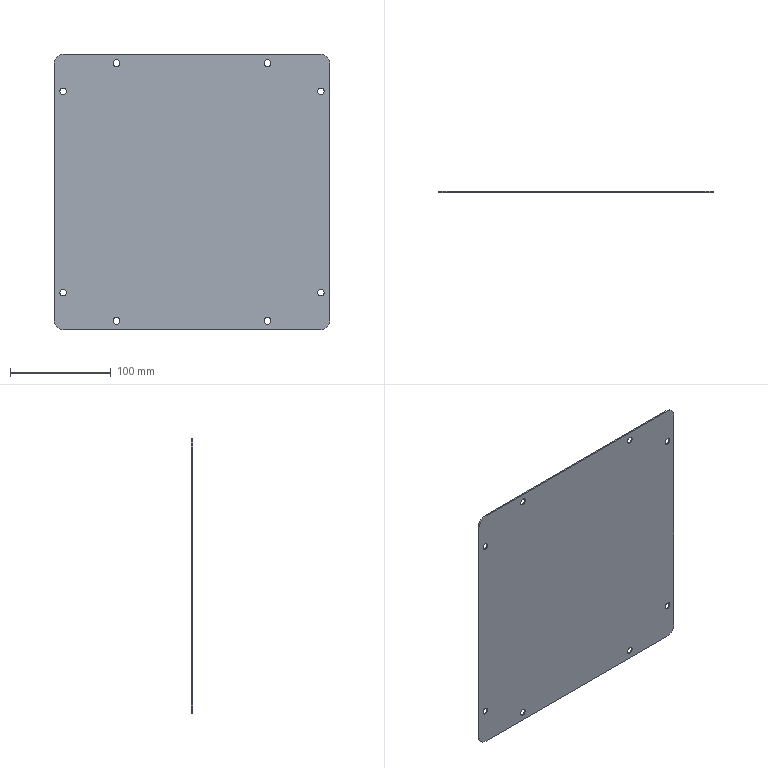Part | STEP file | JBJ-P-1013-05 | 1 solid | 18 faces | box 274 x 1.2 x 274 mm | volume 89670 mm3 | cylinder 12 | plane 6 | commonest cylinder face diameters 6.5 x8 20 x4
STEP:
#1=CARTESIAN_POINT('',(128.,0.,96.75));
#2=VERTEX_POINT('',#1);
#3=CARTESIAN_POINT('',(128.,0.,100.));
#4=DIRECTION('',(0.,-1.,0.));
#5=DIRECTION('',(0.,0.,-1.));
#6=AXIS2_PLACEMENT_3D('',#3,#4,#5);
#7=CIRCLE('',#6,3.25);
#8=EDGE_CURVE('',#2,#2,#7,.T.);
#9=ORIENTED_EDGE('',*,*,#8,.T.);
#10=EDGE_LOOP('',(#9));
#11=FACE_BOUND('',#10,.T.);
#12=CARTESIAN_POINT('',(128.,0.,-103.25));
#13=VERTEX_POINT('',#12);
#14=CARTESIAN_POINT('',(128.,0.,-100.));
#15=DIRECTION('',(0.,-1.,0.));
#16=DIRECTION('',(0.,0.,-1.));
#17=AXIS2_PLACEMENT_3D('',#14,#15,#16);
#18=CIRCLE('',#17,3.25);
#19=EDGE_CURVE('',#13,#13,#18,.T.);
#20=ORIENTED_EDGE('',*,*,#19,.T.);
#21=EDGE_LOOP('',(#20));
#22=FACE_BOUND('',#21,.T.);
#23=CARTESIAN_POINT('',(-128.,0.,-103.25));
#24=VERTEX_POINT('',#23);
#25=CARTESIAN_POINT('',(-128.,0.,-100.));
#26=DIRECTION('',(0.,-1.,0.));
#27=DIRECTION('',(0.,0.,-1.));
#28=AXIS2_PLACEMENT_3D('',#25,#26,#27);
#29=CIRCLE('',#28,3.25);
#30=EDGE_CURVE('',#24,#24,#29,.T.);
#31=ORIENTED_EDGE('',*,*,#30,.T.);
#32=EDGE_LOOP('',(#31));
#33=FACE_BOUND('',#32,.T.);
#34=CARTESIAN_POINT('',(-128.,0.,96.75));
#35=VERTEX_POINT('',#34);
#36=CARTESIAN_POINT('',(-128.,0.,100.));
#37=DIRECTION('',(0.,-1.,0.));
#38=DIRECTION('',(0.,0.,-1.));
#39=AXIS2_PLACEMENT_3D('',#36,#37,#38);
#40=CIRCLE('',#39,3.25);
#41=EDGE_CURVE('',#35,#35,#40,.T.);
#42=ORIENTED_EDGE('',*,*,#41,.T.);
#43=EDGE_LOOP('',(#42));
#44=FACE_BOUND('',#43,.T.);
#45=CARTESIAN_POINT('',(-75.,0.,124.75));
#46=VERTEX_POINT('',#45);
#47=CARTESIAN_POINT('',(-75.,0.,128.));
#48=DIRECTION('',(0.,-1.,0.));
#49=DIRECTION('',(0.,0.,-1.));
#50=AXIS2_PLACEMENT_3D('',#47,#48,#49);
#51=CIRCLE('',#50,3.25);
#52=EDGE_CURVE('',#46,#46,#51,.T.);
#53=ORIENTED_EDGE('',*,*,#52,.T.);
#54=EDGE_LOOP('',(#53));
#55=FACE_BOUND('',#54,.T.);
#56=CARTESIAN_POINT('',(75.,0.,124.75));
#57=VERTEX_POINT('',#56);
#58=CARTESIAN_POINT('',(75.,0.,128.));
#59=DIRECTION('',(0.,-1.,0.));
#60=DIRECTION('',(0.,0.,-1.));
#61=AXIS2_PLACEMENT_3D('',#58,#59,#60);
#62=CIRCLE('',#61,3.25);
#63=EDGE_CURVE('',#57,#57,#62,.T.);
#64=ORIENTED_EDGE('',*,*,#63,.T.);
#65=EDGE_LOOP('',(#64));
#66=FACE_BOUND('',#65,.T.);
#67=CARTESIAN_POINT('',(75.,0.,-131.25));
#68=VERTEX_POINT('',#67);
#69=CARTESIAN_POINT('',(75.,0.,-128.));
#70=DIRECTION('',(0.,-1.,0.));
#71=DIRECTION('',(0.,0.,-1.));
#72=AXIS2_PLACEMENT_3D('',#69,#70,#71);
#73=CIRCLE('',#72,3.25);
#74=EDGE_CURVE('',#68,#68,#73,.T.);
#75=ORIENTED_EDGE('',*,*,#74,.T.);
#76=EDGE_LOOP('',(#75));
#77=FACE_BOUND('',#76,.T.);
#78=CARTESIAN_POINT('',(-127.,0.,137.));
#79=VERTEX_POINT('',#78);
#80=CARTESIAN_POINT('',(127.,0.,137.));
#81=VERTEX_POINT('',#80);
#82=CARTESIAN_POINT('',(-137.,0.,137.));
#83=DIRECTION('',(1.,0.,0.));
#84=VECTOR('',#83,1000.);
#85=LINE('',#82,#84);
#86=EDGE_CURVE('',#79,#81,#85,.T.);
#87=ORIENTED_EDGE('',*,*,#86,.T.);
#88=CARTESIAN_POINT('',(137.,0.,127.));
#89=VERTEX_POINT('',#88);
#90=CARTESIAN_POINT('',(127.,0.,127.));
#91=DIRECTION('',(0.,1.,0.));
#92=DIRECTION('',(0.,0.,1.));
#93=AXIS2_PLACEMENT_3D('',#90,#91,#92);
#94=CIRCLE('',#93,10.);
#95=EDGE_CURVE('',#81,#89,#94,.T.);
#96=ORIENTED_EDGE('',*,*,#95,.T.);
#97=CARTESIAN_POINT('',(137.,0.,-127.));
#98=VERTEX_POINT('',#97);
#99=CARTESIAN_POINT('',(137.,0.,-137.));
#100=DIRECTION('',(0.,0.,-1.));
#101=VECTOR('',#100,1000.);
#102=LINE('',#99,#101);
#103=EDGE_CURVE('',#89,#98,#102,.T.);
#104=ORIENTED_EDGE('',*,*,#103,.T.);
#105=CARTESIAN_POINT('',(127.,0.,-137.));
#106=VERTEX_POINT('',#105);
#107=CARTESIAN_POINT('',(127.,0.,-127.));
#108=DIRECTION('',(0.,1.,0.));
#109=DIRECTION('',(0.,0.,1.));
#110=AXIS2_PLACEMENT_3D('',#107,#108,#109);
#111=CIRCLE('',#110,10.);
#112=EDGE_CURVE('',#98,#106,#111,.T.);
#113=ORIENTED_EDGE('',*,*,#112,.T.);
#114=CARTESIAN_POINT('',(-127.,0.,-137.));
#115=VERTEX_POINT('',#114);
#116=CARTESIAN_POINT('',(-137.,0.,-137.));
#117=DIRECTION('',(-1.,0.,0.));
#118=VECTOR('',#117,1000.);
#119=LINE('',#116,#118);
#120=EDGE_CURVE('',#106,#115,#119,.T.);
#121=ORIENTED_EDGE('',*,*,#120,.T.);
#122=CARTESIAN_POINT('',(-137.,0.,-127.));
#123=VERTEX_POINT('',#122);
#124=CARTESIAN_POINT('',(-127.,0.,-127.));
#125=DIRECTION('',(0.,1.,0.));
#126=DIRECTION('',(0.,0.,1.));
#127=AXIS2_PLACEMENT_3D('',#124,#125,#126);
#128=CIRCLE('',#127,10.);
#129=EDGE_CURVE('',#115,#123,#128,.T.);
#130=ORIENTED_EDGE('',*,*,#129,.T.);
#131=CARTESIAN_POINT('',(-137.,0.,127.));
#132=VERTEX_POINT('',#131);
#133=CARTESIAN_POINT('',(-137.,0.,-137.));
#134=DIRECTION('',(0.,0.,1.));
#135=VECTOR('',#134,1000.);
#136=LINE('',#133,#135);
#137=EDGE_CURVE('',#123,#132,#136,.T.);
#138=ORIENTED_EDGE('',*,*,#137,.T.);
#139=CARTESIAN_POINT('',(-127.,0.,127.));
#140=DIRECTION('',(0.,1.,0.));
#141=DIRECTION('',(0.,0.,1.));
#142=AXIS2_PLACEMENT_3D('',#139,#140,#141);
#143=CIRCLE('',#142,10.);
#144=EDGE_CURVE('',#132,#79,#143,.T.);
#145=ORIENTED_EDGE('',*,*,#144,.T.);
#146=EDGE_LOOP('',(#87,#96,#104,#113,#121,#130,#138,#145));
#147=FACE_OUTER_BOUND('',#146,.T.);
#148=CARTESIAN_POINT('',(-75.,0.,-131.25));
#149=VERTEX_POINT('',#148);
#150=CARTESIAN_POINT('',(-75.,0.,-128.));
#151=DIRECTION('',(0.,-1.,0.));
#152=DIRECTION('',(0.,0.,-1.));
#153=AXIS2_PLACEMENT_3D('',#150,#151,#152);
#154=CIRCLE('',#153,3.25);
#155=EDGE_CURVE('',#149,#149,#154,.T.);
#156=ORIENTED_EDGE('',*,*,#155,.T.);
#157=EDGE_LOOP('',(#156));
#158=FACE_BOUND('',#157,.T.);
#159=CARTESIAN_POINT('',(0.,0.,0.));
#160=DIRECTION('',(0.,1.,0.));
#161=DIRECTION('',(0.,0.,1.));
#162=AXIS2_PLACEMENT_3D('',#159,#160,#161);
#163=PLANE('',#162);
#164=ADVANCED_FACE('',(#11,#22,#33,#44,#55,#66,#77,#147,#158),#163,.T.);
#165=ORIENTED_EDGE('',*,*,#103,.F.);
#166=CARTESIAN_POINT('',(137.,-1.2,127.));
#167=VERTEX_POINT('',#166);
#168=CARTESIAN_POINT('',(137.,-1.2,127.));
#169=DIRECTION('',(0.,-1.,0.));
#170=VECTOR('',#169,1000.);
#171=LINE('',#168,#170);
#172=EDGE_CURVE('',#89,#167,#171,.T.);
#173=ORIENTED_EDGE('',*,*,#172,.T.);
#174=CARTESIAN_POINT('',(137.,-1.2,-127.));
#175=VERTEX_POINT('',#174);
#176=CARTESIAN_POINT('',(137.,-1.2,-137.));
#177=DIRECTION('',(0.,0.,-1.));
#178=VECTOR('',#177,1000.);
#179=LINE('',#176,#178);
#180=EDGE_CURVE('',#167,#175,#179,.T.);
#181=ORIENTED_EDGE('',*,*,#180,.T.);
#182=CARTESIAN_POINT('',(137.,-1.2,-127.));
#183=DIRECTION('',(0.,1.,0.));
#184=VECTOR('',#183,1000.);
#185=LINE('',#182,#184);
#186=EDGE_CURVE('',#175,#98,#185,.T.);
#187=ORIENTED_EDGE('',*,*,#186,.T.);
#188=EDGE_LOOP('',(#165,#173,#181,#187));
#189=FACE_OUTER_BOUND('',#188,.T.);
#190=CARTESIAN_POINT('',(137.,-1.2,-137.));
#191=DIRECTION('',(1.,0.,0.));
#192=DIRECTION('',(0.,0.,-1.));
#193=AXIS2_PLACEMENT_3D('',#190,#191,#192);
#194=PLANE('',#193);
#195=ADVANCED_FACE('',(#189),#194,.T.);
#196=CARTESIAN_POINT('',(-127.,-1.2,137.));
#197=VERTEX_POINT('',#196);
#198=CARTESIAN_POINT('',(127.,-1.2,137.));
#199=VERTEX_POINT('',#198);
#200=CARTESIAN_POINT('',(-137.,-1.2,137.));
#201=DIRECTION('',(1.,0.,0.));
#202=VECTOR('',#201,1000.);
#203=LINE('',#200,#202);
#204=EDGE_CURVE('',#197,#199,#203,.T.);
#205=ORIENTED_EDGE('',*,*,#204,.T.);
#206=CARTESIAN_POINT('',(127.,-1.2,137.));
#207=DIRECTION('',(0.,1.,0.));
#208=VECTOR('',#207,1000.);
#209=LINE('',#206,#208);
#210=EDGE_CURVE('',#199,#81,#209,.T.);
#211=ORIENTED_EDGE('',*,*,#210,.T.);
#212=ORIENTED_EDGE('',*,*,#86,.F.);
#213=CARTESIAN_POINT('',(-127.,-1.2,137.));
#214=DIRECTION('',(0.,-1.,0.));
#215=VECTOR('',#214,1000.);
#216=LINE('',#213,#215);
#217=EDGE_CURVE('',#79,#197,#216,.T.);
#218=ORIENTED_EDGE('',*,*,#217,.T.);
#219=EDGE_LOOP('',(#205,#211,#212,#218));
#220=FACE_OUTER_BOUND('',#219,.T.);
#221=CARTESIAN_POINT('',(-137.,-1.2,137.));
#222=DIRECTION('',(0.,0.,1.));
#223=DIRECTION('',(1.,0.,0.));
#224=AXIS2_PLACEMENT_3D('',#221,#222,#223);
#225=PLANE('',#224);
#226=ADVANCED_FACE('',(#220),#225,.T.);
#227=ORIENTED_EDGE('',*,*,#137,.F.);
#228=CARTESIAN_POINT('',(-137.,-1.2,-127.));
#229=VERTEX_POINT('',#228);
#230=CARTESIAN_POINT('',(-137.,-1.2,-127.));
#231=DIRECTION('',(0.,-1.,0.));
#232=VECTOR('',#231,1000.);
#233=LINE('',#230,#232);
#234=EDGE_CURVE('',#123,#229,#233,.T.);
#235=ORIENTED_EDGE('',*,*,#234,.T.);
#236=CARTESIAN_POINT('',(-137.,-1.2,127.));
#237=VERTEX_POINT('',#236);
#238=CARTESIAN_POINT('',(-137.,-1.2,-137.));
#239=DIRECTION('',(0.,0.,1.));
#240=VECTOR('',#239,1000.);
#241=LINE('',#238,#240);
#242=EDGE_CURVE('',#229,#237,#241,.T.);
#243=ORIENTED_EDGE('',*,*,#242,.T.);
#244=CARTESIAN_POINT('',(-137.,-1.2,127.));
#245=DIRECTION('',(0.,1.,0.));
#246=VECTOR('',#245,1000.);
#247=LINE('',#244,#246);
#248=EDGE_CURVE('',#237,#132,#247,.T.);
#249=ORIENTED_EDGE('',*,*,#248,.T.);
#250=EDGE_LOOP('',(#227,#235,#243,#249));
#251=FACE_OUTER_BOUND('',#250,.T.);
#252=CARTESIAN_POINT('',(-137.,-1.2,-137.));
#253=DIRECTION('',(-1.,0.,0.));
#254=DIRECTION('',(0.,0.,1.));
#255=AXIS2_PLACEMENT_3D('',#252,#253,#254);
#256=PLANE('',#255);
#257=ADVANCED_FACE('',(#251),#256,.T.);
#258=ORIENTED_EDGE('',*,*,#120,.F.);
#259=CARTESIAN_POINT('',(127.,-1.2,-137.));
#260=VERTEX_POINT('',#259);
#261=CARTESIAN_POINT('',(127.,-1.2,-137.));
#262=DIRECTION('',(0.,-1.,0.));
#263=VECTOR('',#262,1000.);
#264=LINE('',#261,#263);
#265=EDGE_CURVE('',#106,#260,#264,.T.);
#266=ORIENTED_EDGE('',*,*,#265,.T.);
#267=CARTESIAN_POINT('',(-127.,-1.2,-137.));
#268=VERTEX_POINT('',#267);
#269=CARTESIAN_POINT('',(-137.,-1.2,-137.));
#270=DIRECTION('',(-1.,0.,0.));
#271=VECTOR('',#270,1000.);
#272=LINE('',#269,#271);
#273=EDGE_CURVE('',#260,#268,#272,.T.);
#274=ORIENTED_EDGE('',*,*,#273,.T.);
#275=CARTESIAN_POINT('',(-127.,-1.2,-137.));
#276=DIRECTION('',(0.,1.,0.));
#277=VECTOR('',#276,1000.);
#278=LINE('',#275,#277);
#279=EDGE_CURVE('',#268,#115,#278,.T.);
#280=ORIENTED_EDGE('',*,*,#279,.T.);
#281=EDGE_LOOP('',(#258,#266,#274,#280));
#282=FACE_OUTER_BOUND('',#281,.T.);
#283=CARTESIAN_POINT('',(-137.,-1.2,-137.));
#284=DIRECTION('',(0.,0.,-1.));
#285=DIRECTION('',(-1.,0.,0.));
#286=AXIS2_PLACEMENT_3D('',#283,#284,#285);
#287=PLANE('',#286);
#288=ADVANCED_FACE('',(#282),#287,.T.);
#289=CARTESIAN_POINT('',(128.,-1.2,96.75));
#290=VERTEX_POINT('',#289);
#291=CARTESIAN_POINT('',(128.,-1.2,100.));
#292=DIRECTION('',(0.,-1.,0.));
#293=DIRECTION('',(0.,0.,-1.));
#294=AXIS2_PLACEMENT_3D('',#291,#292,#293);
#295=CIRCLE('',#294,3.25);
#296=EDGE_CURVE('',#290,#290,#295,.T.);
#297=ORIENTED_EDGE('',*,*,#296,.F.);
#298=EDGE_LOOP('',(#297));
#299=FACE_BOUND('',#298,.T.);
#300=CARTESIAN_POINT('',(128.,-1.2,-103.25));
#301=VERTEX_POINT('',#300);
#302=CARTESIAN_POINT('',(128.,-1.2,-100.));
#303=DIRECTION('',(0.,-1.,0.));
#304=DIRECTION('',(0.,0.,-1.));
#305=AXIS2_PLACEMENT_3D('',#302,#303,#304);
#306=CIRCLE('',#305,3.25);
#307=EDGE_CURVE('',#301,#301,#306,.T.);
#308=ORIENTED_EDGE('',*,*,#307,.F.);
#309=EDGE_LOOP('',(#308));
#310=FACE_BOUND('',#309,.T.);
#311=CARTESIAN_POINT('',(-128.,-1.2,-103.25));
#312=VERTEX_POINT('',#311);
#313=CARTESIAN_POINT('',(-128.,-1.2,-100.));
#314=DIRECTION('',(0.,-1.,0.));
#315=DIRECTION('',(0.,0.,-1.));
#316=AXIS2_PLACEMENT_3D('',#313,#314,#315);
#317=CIRCLE('',#316,3.25);
#318=EDGE_CURVE('',#312,#312,#317,.T.);
#319=ORIENTED_EDGE('',*,*,#318,.F.);
#320=EDGE_LOOP('',(#319));
#321=FACE_BOUND('',#320,.T.);
#322=CARTESIAN_POINT('',(-128.,-1.2,96.75));
#323=VERTEX_POINT('',#322);
#324=CARTESIAN_POINT('',(-128.,-1.2,100.));
#325=DIRECTION('',(0.,-1.,0.));
#326=DIRECTION('',(0.,0.,-1.));
#327=AXIS2_PLACEMENT_3D('',#324,#325,#326);
#328=CIRCLE('',#327,3.25);
#329=EDGE_CURVE('',#323,#323,#328,.T.);
#330=ORIENTED_EDGE('',*,*,#329,.F.);
#331=EDGE_LOOP('',(#330));
#332=FACE_BOUND('',#331,.T.);
#333=CARTESIAN_POINT('',(-75.,-1.2,124.75));
#334=VERTEX_POINT('',#333);
#335=CARTESIAN_POINT('',(-75.,-1.2,128.));
#336=DIRECTION('',(0.,-1.,0.));
#337=DIRECTION('',(0.,0.,-1.));
#338=AXIS2_PLACEMENT_3D('',#335,#336,#337);
#339=CIRCLE('',#338,3.25);
#340=EDGE_CURVE('',#334,#334,#339,.T.);
#341=ORIENTED_EDGE('',*,*,#340,.F.);
#342=EDGE_LOOP('',(#341));
#343=FACE_BOUND('',#342,.T.);
#344=CARTESIAN_POINT('',(75.,-1.2,124.75));
#345=VERTEX_POINT('',#344);
#346=CARTESIAN_POINT('',(75.,-1.2,128.));
#347=DIRECTION('',(0.,-1.,0.));
#348=DIRECTION('',(0.,0.,-1.));
#349=AXIS2_PLACEMENT_3D('',#346,#347,#348);
#350=CIRCLE('',#349,3.25);
#351=EDGE_CURVE('',#345,#345,#350,.T.);
#352=ORIENTED_EDGE('',*,*,#351,.F.);
#353=EDGE_LOOP('',(#352));
#354=FACE_BOUND('',#353,.T.);
#355=CARTESIAN_POINT('',(75.,-1.2,-131.25));
#356=VERTEX_POINT('',#355);
#357=CARTESIAN_POINT('',(75.,-1.2,-128.));
#358=DIRECTION('',(0.,-1.,0.));
#359=DIRECTION('',(0.,0.,-1.));
#360=AXIS2_PLACEMENT_3D('',#357,#358,#359);
#361=CIRCLE('',#360,3.25);
#362=EDGE_CURVE('',#356,#356,#361,.T.);
#363=ORIENTED_EDGE('',*,*,#362,.F.);
#364=EDGE_LOOP('',(#363));
#365=FACE_BOUND('',#364,.T.);
#366=CARTESIAN_POINT('',(-75.,-1.2,-131.25));
#367=VERTEX_POINT('',#366);
#368=CARTESIAN_POINT('',(-75.,-1.2,-128.));
#369=DIRECTION('',(0.,-1.,0.));
#370=DIRECTION('',(0.,0.,-1.));
#371=AXIS2_PLACEMENT_3D('',#368,#369,#370);
#372=CIRCLE('',#371,3.25);
#373=EDGE_CURVE('',#367,#367,#372,.T.);
#374=ORIENTED_EDGE('',*,*,#373,.F.);
#375=EDGE_LOOP('',(#374));
#376=FACE_BOUND('',#375,.T.);
#377=ORIENTED_EDGE('',*,*,#180,.F.);
#378=CARTESIAN_POINT('',(127.,-1.2,127.));
#379=DIRECTION('',(0.,-1.,0.));
#380=DIRECTION('',(0.,0.,1.));
#381=AXIS2_PLACEMENT_3D('',#378,#379,#380);
#382=CIRCLE('',#381,10.);
#383=EDGE_CURVE('',#167,#199,#382,.T.);
#384=ORIENTED_EDGE('',*,*,#383,.T.);
#385=ORIENTED_EDGE('',*,*,#204,.F.);
#386=CARTESIAN_POINT('',(-127.,-1.2,127.));
#387=DIRECTION('',(0.,-1.,0.));
#388=DIRECTION('',(0.,0.,1.));
#389=AXIS2_PLACEMENT_3D('',#386,#387,#388);
#390=CIRCLE('',#389,10.);
#391=EDGE_CURVE('',#197,#237,#390,.T.);
#392=ORIENTED_EDGE('',*,*,#391,.T.);
#393=ORIENTED_EDGE('',*,*,#242,.F.);
#394=CARTESIAN_POINT('',(-127.,-1.2,-127.));
#395=DIRECTION('',(0.,-1.,0.));
#396=DIRECTION('',(0.,0.,1.));
#397=AXIS2_PLACEMENT_3D('',#394,#395,#396);
#398=CIRCLE('',#397,10.);
#399=EDGE_CURVE('',#229,#268,#398,.T.);
#400=ORIENTED_EDGE('',*,*,#399,.T.);
#401=ORIENTED_EDGE('',*,*,#273,.F.);
#402=CARTESIAN_POINT('',(127.,-1.2,-127.));
#403=DIRECTION('',(0.,-1.,0.));
#404=DIRECTION('',(0.,0.,1.));
#405=AXIS2_PLACEMENT_3D('',#402,#403,#404);
#406=CIRCLE('',#405,10.);
#407=EDGE_CURVE('',#260,#175,#406,.T.);
#408=ORIENTED_EDGE('',*,*,#407,.T.);
#409=EDGE_LOOP('',(#377,#384,#385,#392,#393,#400,#401,#408));
#410=FACE_OUTER_BOUND('',#409,.T.);
#411=CARTESIAN_POINT('',(0.,-1.2,0.));
#412=DIRECTION('',(0.,1.,0.));
#413=DIRECTION('',(0.,0.,1.));
#414=AXIS2_PLACEMENT_3D('',#411,#412,#413);
#415=PLANE('',#414);
#416=ADVANCED_FACE('',(#299,#310,#321,#332,#343,#354,#365,#376,#410),#415,.F.);
#417=ORIENTED_EDGE('',*,*,#383,.F.);
#418=ORIENTED_EDGE('',*,*,#172,.F.);
#419=ORIENTED_EDGE('',*,*,#95,.F.);
#420=ORIENTED_EDGE('',*,*,#210,.F.);
#421=EDGE_LOOP('',(#417,#418,#419,#420));
#422=FACE_OUTER_BOUND('',#421,.T.);
#423=CARTESIAN_POINT('',(127.,-1.2,127.));
#424=DIRECTION('',(0.,1.,0.));
#425=DIRECTION('',(0.,0.,1.));
#426=AXIS2_PLACEMENT_3D('',#423,#424,#425);
#427=CYLINDRICAL_SURFACE('',#426,10.);
#428=ADVANCED_FACE('',(#422),#427,.T.);
#429=ORIENTED_EDGE('',*,*,#407,.F.);
#430=ORIENTED_EDGE('',*,*,#265,.F.);
#431=ORIENTED_EDGE('',*,*,#112,.F.);
#432=ORIENTED_EDGE('',*,*,#186,.F.);
#433=EDGE_LOOP('',(#429,#430,#431,#432));
#434=FACE_OUTER_BOUND('',#433,.T.);
#435=CARTESIAN_POINT('',(127.,-1.2,-127.));
#436=DIRECTION('',(0.,1.,0.));
#437=DIRECTION('',(0.,0.,1.));
#438=AXIS2_PLACEMENT_3D('',#435,#436,#437);
#439=CYLINDRICAL_SURFACE('',#438,10.);
#440=ADVANCED_FACE('',(#434),#439,.T.);
#441=ORIENTED_EDGE('',*,*,#399,.F.);
#442=ORIENTED_EDGE('',*,*,#234,.F.);
#443=ORIENTED_EDGE('',*,*,#129,.F.);
#444=ORIENTED_EDGE('',*,*,#279,.F.);
#445=EDGE_LOOP('',(#441,#442,#443,#444));
#446=FACE_OUTER_BOUND('',#445,.T.);
#447=CARTESIAN_POINT('',(-127.,-1.2,-127.));
#448=DIRECTION('',(0.,1.,0.));
#449=DIRECTION('',(0.,0.,1.));
#450=AXIS2_PLACEMENT_3D('',#447,#448,#449);
#451=CYLINDRICAL_SURFACE('',#450,10.);
#452=ADVANCED_FACE('',(#446),#451,.T.);
#453=ORIENTED_EDGE('',*,*,#391,.F.);
#454=ORIENTED_EDGE('',*,*,#217,.F.);
#455=ORIENTED_EDGE('',*,*,#144,.F.);
#456=ORIENTED_EDGE('',*,*,#248,.F.);
#457=EDGE_LOOP('',(#453,#454,#455,#456));
#458=FACE_OUTER_BOUND('',#457,.T.);
#459=CARTESIAN_POINT('',(-127.,-1.2,127.));
#460=DIRECTION('',(0.,1.,0.));
#461=DIRECTION('',(0.,0.,1.));
#462=AXIS2_PLACEMENT_3D('',#459,#460,#461);
#463=CYLINDRICAL_SURFACE('',#462,10.);
#464=ADVANCED_FACE('',(#458),#463,.T.);
#465=ORIENTED_EDGE('',*,*,#155,.F.);
#466=EDGE_LOOP('',(#465));
#467=FACE_OUTER_BOUND('',#466,.T.);
#468=ORIENTED_EDGE('',*,*,#373,.T.);
#469=EDGE_LOOP('',(#468));
#470=FACE_OUTER_BOUND('',#469,.T.);
#471=CARTESIAN_POINT('',(-75.,-1.2,-128.));
#472=DIRECTION('',(0.,-1.,0.));
#473=DIRECTION('',(0.,0.,-1.));
#474=AXIS2_PLACEMENT_3D('',#471,#472,#473);
#475=CYLINDRICAL_SURFACE('',#474,3.25);
#476=ADVANCED_FACE('',(#467,#470),#475,.F.);
#477=ORIENTED_EDGE('',*,*,#74,.F.);
#478=EDGE_LOOP('',(#477));
#479=FACE_OUTER_BOUND('',#478,.T.);
#480=ORIENTED_EDGE('',*,*,#362,.T.);
#481=EDGE_LOOP('',(#480));
#482=FACE_OUTER_BOUND('',#481,.T.);
#483=CARTESIAN_POINT('',(75.,-1.2,-128.));
#484=DIRECTION('',(0.,-1.,0.));
#485=DIRECTION('',(0.,0.,-1.));
#486=AXIS2_PLACEMENT_3D('',#483,#484,#485);
#487=CYLINDRICAL_SURFACE('',#486,3.25);
#488=ADVANCED_FACE('',(#479,#482),#487,.F.);
#489=ORIENTED_EDGE('',*,*,#63,.F.);
#490=EDGE_LOOP('',(#489));
#491=FACE_OUTER_BOUND('',#490,.T.);
#492=ORIENTED_EDGE('',*,*,#351,.T.);
#493=EDGE_LOOP('',(#492));
#494=FACE_OUTER_BOUND('',#493,.T.);
#495=CARTESIAN_POINT('',(75.,-1.2,128.));
#496=DIRECTION('',(0.,-1.,0.));
#497=DIRECTION('',(0.,0.,-1.));
#498=AXIS2_PLACEMENT_3D('',#495,#496,#497);
#499=CYLINDRICAL_SURFACE('',#498,3.25);
#500=ADVANCED_FACE('',(#491,#494),#499,.F.);
#501=ORIENTED_EDGE('',*,*,#52,.F.);
#502=EDGE_LOOP('',(#501));
#503=FACE_OUTER_BOUND('',#502,.T.);
#504=ORIENTED_EDGE('',*,*,#340,.T.);
#505=EDGE_LOOP('',(#504));
#506=FACE_OUTER_BOUND('',#505,.T.);
#507=CARTESIAN_POINT('',(-75.,-1.2,128.));
#508=DIRECTION('',(0.,-1.,0.));
#509=DIRECTION('',(0.,0.,-1.));
#510=AXIS2_PLACEMENT_3D('',#507,#508,#509);
#511=CYLINDRICAL_SURFACE('',#510,3.25);
#512=ADVANCED_FACE('',(#503,#506),#511,.F.);
#513=ORIENTED_EDGE('',*,*,#41,.F.);
#514=EDGE_LOOP('',(#513));
#515=FACE_OUTER_BOUND('',#514,.T.);
#516=ORIENTED_EDGE('',*,*,#329,.T.);
#517=EDGE_LOOP('',(#516));
#518=FACE_OUTER_BOUND('',#517,.T.);
#519=CARTESIAN_POINT('',(-128.,-1.2,100.));
#520=DIRECTION('',(0.,-1.,0.));
#521=DIRECTION('',(0.,0.,-1.));
#522=AXIS2_PLACEMENT_3D('',#519,#520,#521);
#523=CYLINDRICAL_SURFACE('',#522,3.25);
#524=ADVANCED_FACE('',(#515,#518),#523,.F.);
#525=ORIENTED_EDGE('',*,*,#30,.F.);
#526=EDGE_LOOP('',(#525));
#527=FACE_OUTER_BOUND('',#526,.T.);
#528=ORIENTED_EDGE('',*,*,#318,.T.);
#529=EDGE_LOOP('',(#528));
#530=FACE_OUTER_BOUND('',#529,.T.);
#531=CARTESIAN_POINT('',(-128.,-1.2,-100.));
#532=DIRECTION('',(0.,-1.,0.));
#533=DIRECTION('',(0.,0.,-1.));
#534=AXIS2_PLACEMENT_3D('',#531,#532,#533);
#535=CYLINDRICAL_SURFACE('',#534,3.25);
#536=ADVANCED_FACE('',(#527,#530),#535,.F.);
#537=ORIENTED_EDGE('',*,*,#19,.F.);
#538=EDGE_LOOP('',(#537));
#539=FACE_OUTER_BOUND('',#538,.T.);
#540=ORIENTED_EDGE('',*,*,#307,.T.);
#541=EDGE_LOOP('',(#540));
#542=FACE_OUTER_BOUND('',#541,.T.);
#543=CARTESIAN_POINT('',(128.,-1.2,-100.));
#544=DIRECTION('',(0.,-1.,0.));
#545=DIRECTION('',(0.,0.,-1.));
#546=AXIS2_PLACEMENT_3D('',#543,#544,#545);
#547=CYLINDRICAL_SURFACE('',#546,3.25);
#548=ADVANCED_FACE('',(#539,#542),#547,.F.);
#549=ORIENTED_EDGE('',*,*,#8,.F.);
#550=EDGE_LOOP('',(#549));
#551=FACE_OUTER_BOUND('',#550,.T.);
#552=ORIENTED_EDGE('',*,*,#296,.T.);
#553=EDGE_LOOP('',(#552));
#554=FACE_OUTER_BOUND('',#553,.T.);
#555=CARTESIAN_POINT('',(128.,-1.2,100.));
#556=DIRECTION('',(0.,-1.,0.));
#557=DIRECTION('',(0.,0.,-1.));
#558=AXIS2_PLACEMENT_3D('',#555,#556,#557);
#559=CYLINDRICAL_SURFACE('',#558,3.25);
#560=ADVANCED_FACE('',(#551,#554),#559,.F.);
#561=CLOSED_SHELL('',(#164,#195,#226,#257,#288,#416,#428,#440,#452,#464,#476,#488,#500,#512,#524,#536,#548,#560));
#562=MANIFOLD_SOLID_BREP('',#561);
#563=CARTESIAN_POINT('',(0.,0.,0.));
#564=DIRECTION('',(0.,0.,1.));
#565=DIRECTION('',(1.,0.,0.));
#566=AXIS2_PLACEMENT_3D('',#563,#564,#565);
#567=(LENGTH_UNIT()NAMED_UNIT(*)SI_UNIT(.MILLI.,.METRE.));
#568=UNCERTAINTY_MEASURE_WITH_UNIT(LENGTH_MEASURE(0.00001),#567,'','');
#569=(NAMED_UNIT(*)PLANE_ANGLE_UNIT()SI_UNIT($,.RADIAN.));
#570=(NAMED_UNIT(*)SI_UNIT($,.STERADIAN.)SOLID_ANGLE_UNIT());
#571=(GEOMETRIC_REPRESENTATION_CONTEXT(3)GLOBAL_UNCERTAINTY_ASSIGNED_CONTEXT((#568))GLOBAL_UNIT_ASSIGNED_CONTEXT((#567,#569,#570))REPRESENTATION_CONTEXT('',''));
#572=ADVANCED_BREP_SHAPE_REPRESENTATION('',(#562,#566),#571);